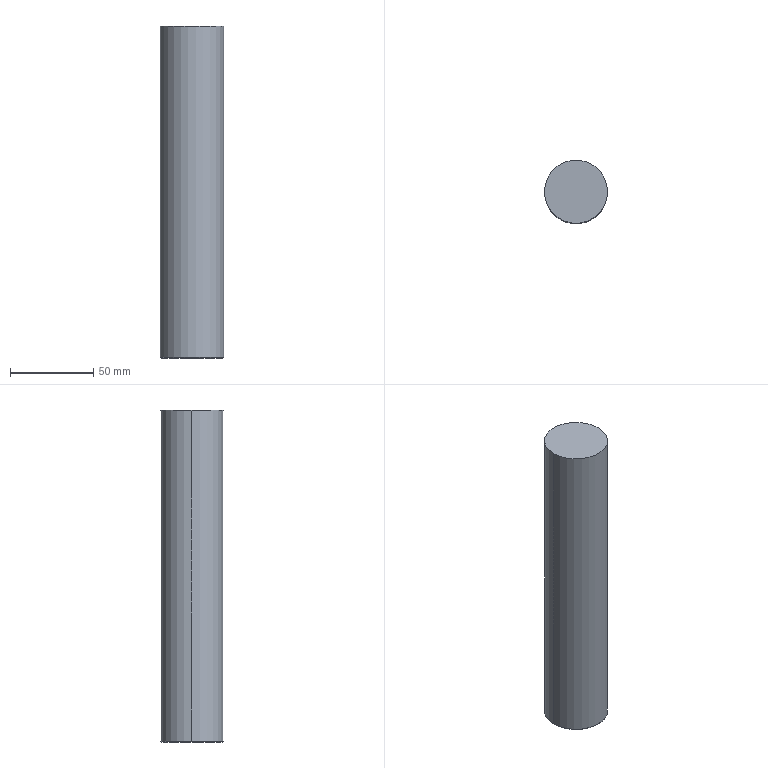Part | NX | features MYKP38-200_3 2 | 1 solid | 6 faces | box 38 x 38 x 200 mm | volume 226808 mm3 | cone 2 | plane 2 | cylinder 2 | commonest cylinder face diameters 38 x2
STEP:
#1=CARTESIAN_POINT('',(1741.477,-312.405,-150.001));
#2=VERTEX_POINT('',#1);
#3=CARTESIAN_POINT('',(1740.977,-312.405,-149.501));
#4=VERTEX_POINT('',#3);
#5=CARTESIAN_POINT('',(1741.477,-312.405,-150.001));
#6=DIRECTION('',(-0.7071,-0.000000003,0.7071));
#7=VECTOR('',#6,1000.);
#8=LINE('',#5,#7);
#9=EDGE_CURVE('',#2,#4,#8,.T.);
#10=ORIENTED_EDGE('',*,*,#9,.F.);
#11=CARTESIAN_POINT('',(1778.477,-312.405,-150.001));
#12=VERTEX_POINT('',#11);
#13=CARTESIAN_POINT('',(1759.977,-312.405,-150.001));
#14=DIRECTION('',(0.,0.,1.));
#15=DIRECTION('',(-1.,0.,0.));
#16=AXIS2_PLACEMENT_3D('',#13,#14,#15);
#17=CIRCLE('',#16,18.5);
#18=EDGE_CURVE('',#2,#12,#17,.T.);
#19=ORIENTED_EDGE('',*,*,#18,.T.);
#20=CARTESIAN_POINT('',(1778.977,-312.405,-149.501));
#21=VERTEX_POINT('',#20);
#22=CARTESIAN_POINT('',(1778.477,-312.405,-150.001));
#23=DIRECTION('',(0.7071,0.000000003,0.7071));
#24=VECTOR('',#23,1000.);
#25=LINE('',#22,#24);
#26=EDGE_CURVE('',#21,#12,#25,.F.);
#27=ORIENTED_EDGE('',*,*,#26,.F.);
#28=CARTESIAN_POINT('',(1759.977,-312.405,-149.501));
#29=DIRECTION('',(0.,0.,1.));
#30=DIRECTION('',(-1.,0.,0.));
#31=AXIS2_PLACEMENT_3D('',#28,#29,#30);
#32=CIRCLE('',#31,19.);
#33=EDGE_CURVE('',#4,#21,#32,.T.);
#34=ORIENTED_EDGE('',*,*,#33,.F.);
#35=EDGE_LOOP('',(#10,#19,#27,#34));
#36=FACE_BOUND('',#35,.T.);
#37=CARTESIAN_POINT('',(1759.977,-312.405,-149.751));
#38=DIRECTION('',(0.,0.,1.));
#39=DIRECTION('',(0.,-1.,0.));
#40=AXIS2_PLACEMENT_3D('',#37,#38,#39);
#41=CONICAL_SURFACE('',#40,18.75,0.7854);
#42=ADVANCED_FACE('',(#36),#41,.T.);
#43=ORIENTED_EDGE('',*,*,#26,.T.);
#44=CARTESIAN_POINT('',(1759.977,-312.405,-150.001));
#45=DIRECTION('',(0.,0.,1.));
#46=DIRECTION('',(1.,0.,0.));
#47=AXIS2_PLACEMENT_3D('',#44,#45,#46);
#48=CIRCLE('',#47,18.5);
#49=EDGE_CURVE('',#12,#2,#48,.T.);
#50=ORIENTED_EDGE('',*,*,#49,.T.);
#51=ORIENTED_EDGE('',*,*,#9,.T.);
#52=CARTESIAN_POINT('',(1759.977,-312.405,-149.501));
#53=DIRECTION('',(0.,0.,1.));
#54=DIRECTION('',(1.,0.,0.));
#55=AXIS2_PLACEMENT_3D('',#52,#53,#54);
#56=CIRCLE('',#55,19.);
#57=EDGE_CURVE('',#21,#4,#56,.T.);
#58=ORIENTED_EDGE('',*,*,#57,.F.);
#59=EDGE_LOOP('',(#43,#50,#51,#58));
#60=FACE_BOUND('',#59,.T.);
#61=CARTESIAN_POINT('',(1759.977,-312.405,-149.751));
#62=DIRECTION('',(0.,0.,1.));
#63=DIRECTION('',(0.,-1.,0.));
#64=AXIS2_PLACEMENT_3D('',#61,#62,#63);
#65=CONICAL_SURFACE('',#64,18.75,0.7854);
#66=ADVANCED_FACE('',(#60),#65,.T.);
#67=ORIENTED_EDGE('',*,*,#18,.F.);
#68=ORIENTED_EDGE('',*,*,#49,.F.);
#69=EDGE_LOOP('',(#67,#68));
#70=FACE_BOUND('',#69,.T.);
#71=CARTESIAN_POINT('',(1759.977,-312.405,-150.001));
#72=DIRECTION('',(0.,0.,-1.));
#73=DIRECTION('',(1.,0.,0.));
#74=AXIS2_PLACEMENT_3D('',#71,#72,#73);
#75=PLANE('',#74);
#76=ADVANCED_FACE('',(#70),#75,.T.);
#77=CARTESIAN_POINT('',(1740.977,-312.405,-3.001));
#78=VERTEX_POINT('',#77);
#79=CARTESIAN_POINT('',(1740.977,-312.405,49.999));
#80=VERTEX_POINT('',#79);
#81=CARTESIAN_POINT('',(1740.977,-312.405,-79.501));
#82=DIRECTION('',(-0.000000019,0.,1.));
#83=VECTOR('',#82,1000.);
#84=LINE('',#81,#83);
#85=EDGE_CURVE('',#78,#80,#84,.T.);
#86=ORIENTED_EDGE('',*,*,#85,.T.);
#87=CARTESIAN_POINT('',(1778.977,-312.405,49.999));
#88=VERTEX_POINT('',#87);
#89=CARTESIAN_POINT('',(1759.977,-312.405,49.999));
#90=DIRECTION('',(0.,0.,-1.));
#91=DIRECTION('',(-1.,0.,0.));
#92=AXIS2_PLACEMENT_3D('',#89,#90,#91);
#93=CIRCLE('',#92,19.);
#94=EDGE_CURVE('',#80,#88,#93,.T.);
#95=ORIENTED_EDGE('',*,*,#94,.T.);
#96=CARTESIAN_POINT('',(1778.977,-312.405,-3.001));
#97=VERTEX_POINT('',#96);
#98=CARTESIAN_POINT('',(1778.977,-312.405,-79.501));
#99=DIRECTION('',(0.000000019,0.,1.));
#100=VECTOR('',#99,1000.);
#101=LINE('',#98,#100);
#102=EDGE_CURVE('',#88,#97,#101,.F.);
#103=ORIENTED_EDGE('',*,*,#102,.T.);
#104=CARTESIAN_POINT('',(1778.977,-312.405,-5.001));
#105=VERTEX_POINT('',#104);
#106=CARTESIAN_POINT('',(1778.977,-312.405,-79.501));
#107=DIRECTION('',(0.000000019,0.,1.));
#108=VECTOR('',#107,1000.);
#109=LINE('',#106,#108);
#110=EDGE_CURVE('',#97,#105,#109,.F.);
#111=ORIENTED_EDGE('',*,*,#110,.T.);
#112=CARTESIAN_POINT('',(1778.977,-312.405,-7.001));
#113=VERTEX_POINT('',#112);
#114=CARTESIAN_POINT('',(1778.977,-312.405,-81.501));
#115=DIRECTION('',(0.000000019,0.,1.));
#116=VECTOR('',#115,1000.);
#117=LINE('',#114,#116);
#118=EDGE_CURVE('',#105,#113,#117,.F.);
#119=ORIENTED_EDGE('',*,*,#118,.T.);
#120=CARTESIAN_POINT('',(1778.977,-312.405,-9.001));
#121=VERTEX_POINT('',#120);
#122=CARTESIAN_POINT('',(1778.977,-312.405,-83.501));
#123=DIRECTION('',(0.000000019,0.,1.));
#124=VECTOR('',#123,1000.);
#125=LINE('',#122,#124);
#126=EDGE_CURVE('',#113,#121,#125,.F.);
#127=ORIENTED_EDGE('',*,*,#126,.T.);
#128=CARTESIAN_POINT('',(1778.977,-312.405,-11.001));
#129=VERTEX_POINT('',#128);
#130=CARTESIAN_POINT('',(1778.977,-312.405,-85.501));
#131=DIRECTION('',(0.000000019,0.,1.));
#132=VECTOR('',#131,1000.);
#133=LINE('',#130,#132);
#134=EDGE_CURVE('',#121,#129,#133,.F.);
#135=ORIENTED_EDGE('',*,*,#134,.T.);
#136=CARTESIAN_POINT('',(1778.977,-312.405,-13.001));
#137=VERTEX_POINT('',#136);
#138=CARTESIAN_POINT('',(1778.977,-312.405,-87.501));
#139=DIRECTION('',(0.000000019,0.,1.));
#140=VECTOR('',#139,1000.);
#141=LINE('',#138,#140);
#142=EDGE_CURVE('',#129,#137,#141,.F.);
#143=ORIENTED_EDGE('',*,*,#142,.T.);
#144=CARTESIAN_POINT('',(1778.977,-312.405,-15.001));
#145=VERTEX_POINT('',#144);
#146=CARTESIAN_POINT('',(1778.977,-312.405,-89.501));
#147=DIRECTION('',(0.000000019,0.,1.));
#148=VECTOR('',#147,1000.);
#149=LINE('',#146,#148);
#150=EDGE_CURVE('',#137,#145,#149,.F.);
#151=ORIENTED_EDGE('',*,*,#150,.T.);
#152=CARTESIAN_POINT('',(1778.977,-312.405,-17.001));
#153=VERTEX_POINT('',#152);
#154=CARTESIAN_POINT('',(1778.977,-312.405,-91.501));
#155=DIRECTION('',(0.000000019,0.,1.));
#156=VECTOR('',#155,1000.);
#157=LINE('',#154,#156);
#158=EDGE_CURVE('',#145,#153,#157,.F.);
#159=ORIENTED_EDGE('',*,*,#158,.T.);
#160=CARTESIAN_POINT('',(1778.977,-312.405,-19.001));
#161=VERTEX_POINT('',#160);
#162=CARTESIAN_POINT('',(1778.977,-312.405,-93.501));
#163=DIRECTION('',(0.000000019,0.,1.));
#164=VECTOR('',#163,1000.);
#165=LINE('',#162,#164);
#166=EDGE_CURVE('',#153,#161,#165,.F.);
#167=ORIENTED_EDGE('',*,*,#166,.T.);
#168=CARTESIAN_POINT('',(1778.977,-312.405,-21.001));
#169=VERTEX_POINT('',#168);
#170=CARTESIAN_POINT('',(1778.977,-312.405,-95.501));
#171=DIRECTION('',(0.000000019,0.,1.));
#172=VECTOR('',#171,1000.);
#173=LINE('',#170,#172);
#174=EDGE_CURVE('',#161,#169,#173,.F.);
#175=ORIENTED_EDGE('',*,*,#174,.T.);
#176=CARTESIAN_POINT('',(1778.977,-312.405,-23.001));
#177=VERTEX_POINT('',#176);
#178=CARTESIAN_POINT('',(1778.977,-312.405,-97.501));
#179=DIRECTION('',(0.000000019,0.,1.));
#180=VECTOR('',#179,1000.);
#181=LINE('',#178,#180);
#182=EDGE_CURVE('',#169,#177,#181,.F.);
#183=ORIENTED_EDGE('',*,*,#182,.T.);
#184=CARTESIAN_POINT('',(1778.977,-312.405,-25.001));
#185=VERTEX_POINT('',#184);
#186=CARTESIAN_POINT('',(1778.977,-312.405,-99.501));
#187=DIRECTION('',(0.000000019,0.,1.));
#188=VECTOR('',#187,1000.);
#189=LINE('',#186,#188);
#190=EDGE_CURVE('',#177,#185,#189,.F.);
#191=ORIENTED_EDGE('',*,*,#190,.T.);
#192=CARTESIAN_POINT('',(1778.977,-312.405,-27.001));
#193=VERTEX_POINT('',#192);
#194=CARTESIAN_POINT('',(1778.977,-312.405,-101.501));
#195=DIRECTION('',(0.000000019,0.,1.));
#196=VECTOR('',#195,1000.);
#197=LINE('',#194,#196);
#198=EDGE_CURVE('',#185,#193,#197,.F.);
#199=ORIENTED_EDGE('',*,*,#198,.T.);
#200=CARTESIAN_POINT('',(1778.977,-312.405,-29.001));
#201=VERTEX_POINT('',#200);
#202=CARTESIAN_POINT('',(1778.977,-312.405,-103.501));
#203=DIRECTION('',(0.000000019,0.,1.));
#204=VECTOR('',#203,1000.);
#205=LINE('',#202,#204);
#206=EDGE_CURVE('',#193,#201,#205,.F.);
#207=ORIENTED_EDGE('',*,*,#206,.T.);
#208=CARTESIAN_POINT('',(1778.977,-312.405,-31.001));
#209=VERTEX_POINT('',#208);
#210=CARTESIAN_POINT('',(1778.977,-312.405,-105.501));
#211=DIRECTION('',(0.000000019,0.,1.));
#212=VECTOR('',#211,1000.);
#213=LINE('',#210,#212);
#214=EDGE_CURVE('',#201,#209,#213,.F.);
#215=ORIENTED_EDGE('',*,*,#214,.T.);
#216=CARTESIAN_POINT('',(1778.977,-312.405,-33.001));
#217=VERTEX_POINT('',#216);
#218=CARTESIAN_POINT('',(1778.977,-312.405,-107.501));
#219=DIRECTION('',(0.000000019,0.,1.));
#220=VECTOR('',#219,1000.);
#221=LINE('',#218,#220);
#222=EDGE_CURVE('',#209,#217,#221,.F.);
#223=ORIENTED_EDGE('',*,*,#222,.T.);
#224=CARTESIAN_POINT('',(1778.977,-312.405,-35.001));
#225=VERTEX_POINT('',#224);
#226=CARTESIAN_POINT('',(1778.977,-312.405,-109.501));
#227=DIRECTION('',(0.000000019,0.,1.));
#228=VECTOR('',#227,1000.);
#229=LINE('',#226,#228);
#230=EDGE_CURVE('',#217,#225,#229,.F.);
#231=ORIENTED_EDGE('',*,*,#230,.T.);
#232=CARTESIAN_POINT('',(1778.977,-312.405,-37.001));
#233=VERTEX_POINT('',#232);
#234=CARTESIAN_POINT('',(1778.977,-312.405,-111.501));
#235=DIRECTION('',(0.000000019,0.,1.));
#236=VECTOR('',#235,1000.);
#237=LINE('',#234,#236);
#238=EDGE_CURVE('',#225,#233,#237,.F.);
#239=ORIENTED_EDGE('',*,*,#238,.T.);
#240=CARTESIAN_POINT('',(1778.977,-312.405,-39.001));
#241=VERTEX_POINT('',#240);
#242=CARTESIAN_POINT('',(1778.977,-312.405,-113.501));
#243=DIRECTION('',(0.000000019,0.,1.));
#244=VECTOR('',#243,1000.);
#245=LINE('',#242,#244);
#246=EDGE_CURVE('',#233,#241,#245,.F.);
#247=ORIENTED_EDGE('',*,*,#246,.T.);
#248=CARTESIAN_POINT('',(1778.977,-312.405,-41.001));
#249=VERTEX_POINT('',#248);
#250=CARTESIAN_POINT('',(1778.977,-312.405,-115.501));
#251=DIRECTION('',(0.000000019,0.,1.));
#252=VECTOR('',#251,1000.);
#253=LINE('',#250,#252);
#254=EDGE_CURVE('',#241,#249,#253,.F.);
#255=ORIENTED_EDGE('',*,*,#254,.T.);
#256=CARTESIAN_POINT('',(1778.977,-312.405,-43.001));
#257=VERTEX_POINT('',#256);
#258=CARTESIAN_POINT('',(1778.977,-312.405,-117.501));
#259=DIRECTION('',(0.000000019,0.,1.));
#260=VECTOR('',#259,1000.);
#261=LINE('',#258,#260);
#262=EDGE_CURVE('',#249,#257,#261,.F.);
#263=ORIENTED_EDGE('',*,*,#262,.T.);
#264=CARTESIAN_POINT('',(1778.977,-312.405,-45.001));
#265=VERTEX_POINT('',#264);
#266=CARTESIAN_POINT('',(1778.977,-312.405,-119.501));
#267=DIRECTION('',(0.000000019,0.,1.));
#268=VECTOR('',#267,1000.);
#269=LINE('',#266,#268);
#270=EDGE_CURVE('',#257,#265,#269,.F.);
#271=ORIENTED_EDGE('',*,*,#270,.T.);
#272=CARTESIAN_POINT('',(1778.977,-312.405,-47.001));
#273=VERTEX_POINT('',#272);
#274=CARTESIAN_POINT('',(1778.977,-312.405,-121.501));
#275=DIRECTION('',(0.000000019,0.,1.));
#276=VECTOR('',#275,1000.);
#277=LINE('',#274,#276);
#278=EDGE_CURVE('',#265,#273,#277,.F.);
#279=ORIENTED_EDGE('',*,*,#278,.T.);
#280=CARTESIAN_POINT('',(1778.977,-312.405,-49.001));
#281=VERTEX_POINT('',#280);
#282=CARTESIAN_POINT('',(1778.977,-312.405,-123.501));
#283=DIRECTION('',(0.000000019,0.,1.));
#284=VECTOR('',#283,1000.);
#285=LINE('',#282,#284);
#286=EDGE_CURVE('',#273,#281,#285,.F.);
#287=ORIENTED_EDGE('',*,*,#286,.T.);
#288=CARTESIAN_POINT('',(1778.977,-312.405,-51.001));
#289=VERTEX_POINT('',#288);
#290=CARTESIAN_POINT('',(1778.977,-312.405,-125.501));
#291=DIRECTION('',(0.000000019,0.,1.));
#292=VECTOR('',#291,1000.);
#293=LINE('',#290,#292);
#294=EDGE_CURVE('',#281,#289,#293,.F.);
#295=ORIENTED_EDGE('',*,*,#294,.T.);
#296=CARTESIAN_POINT('',(1778.977,-312.405,-53.001));
#297=VERTEX_POINT('',#296);
#298=CARTESIAN_POINT('',(1778.977,-312.405,-127.501));
#299=DIRECTION('',(0.000000019,0.,1.));
#300=VECTOR('',#299,1000.);
#301=LINE('',#298,#300);
#302=EDGE_CURVE('',#289,#297,#301,.F.);
#303=ORIENTED_EDGE('',*,*,#302,.T.);
#304=CARTESIAN_POINT('',(1778.977,-312.405,-55.001));
#305=VERTEX_POINT('',#304);
#306=CARTESIAN_POINT('',(1778.977,-312.405,-129.501));
#307=DIRECTION('',(0.000000019,0.,1.));
#308=VECTOR('',#307,1000.);
#309=LINE('',#306,#308);
#310=EDGE_CURVE('',#297,#305,#309,.F.);
#311=ORIENTED_EDGE('',*,*,#310,.T.);
#312=CARTESIAN_POINT('',(1778.977,-312.405,-57.001));
#313=VERTEX_POINT('',#312);
#314=CARTESIAN_POINT('',(1778.977,-312.405,-131.501));
#315=DIRECTION('',(0.000000019,0.,1.));
#316=VECTOR('',#315,1000.);
#317=LINE('',#314,#316);
#318=EDGE_CURVE('',#305,#313,#317,.F.);
#319=ORIENTED_EDGE('',*,*,#318,.T.);
#320=CARTESIAN_POINT('',(1778.977,-312.405,-59.001));
#321=VERTEX_POINT('',#320);
#322=CARTESIAN_POINT('',(1778.977,-312.405,-133.501));
#323=DIRECTION('',(0.000000019,0.,1.));
#324=VECTOR('',#323,1000.);
#325=LINE('',#322,#324);
#326=EDGE_CURVE('',#313,#321,#325,.F.);
#327=ORIENTED_EDGE('',*,*,#326,.T.);
#328=CARTESIAN_POINT('',(1778.977,-312.405,-61.001));
#329=VERTEX_POINT('',#328);
#330=CARTESIAN_POINT('',(1778.977,-312.405,-135.501));
#331=DIRECTION('',(0.000000019,0.,1.));
#332=VECTOR('',#331,1000.);
#333=LINE('',#330,#332);
#334=EDGE_CURVE('',#321,#329,#333,.F.);
#335=ORIENTED_EDGE('',*,*,#334,.T.);
#336=CARTESIAN_POINT('',(1778.977,-312.405,-63.001));
#337=VERTEX_POINT('',#336);
#338=CARTESIAN_POINT('',(1778.977,-312.405,-137.501));
#339=DIRECTION('',(0.000000019,0.,1.));
#340=VECTOR('',#339,1000.);
#341=LINE('',#338,#340);
#342=EDGE_CURVE('',#329,#337,#341,.F.);
#343=ORIENTED_EDGE('',*,*,#342,.T.);
#344=CARTESIAN_POINT('',(1778.977,-312.405,-65.001));
#345=VERTEX_POINT('',#344);
#346=CARTESIAN_POINT('',(1778.977,-312.405,-139.501));
#347=DIRECTION('',(0.000000019,0.,1.));
#348=VECTOR('',#347,1000.);
#349=LINE('',#346,#348);
#350=EDGE_CURVE('',#337,#345,#349,.F.);
#351=ORIENTED_EDGE('',*,*,#350,.T.);
#352=CARTESIAN_POINT('',(1778.977,-312.405,-67.001));
#353=VERTEX_POINT('',#352);
#354=CARTESIAN_POINT('',(1778.977,-312.405,-141.501));
#355=DIRECTION('',(0.000000019,0.,1.));
#356=VECTOR('',#355,1000.);
#357=LINE('',#354,#356);
#358=EDGE_CURVE('',#345,#353,#357,.F.);
#359=ORIENTED_EDGE('',*,*,#358,.T.);
#360=CARTESIAN_POINT('',(1778.977,-312.405,-69.001));
#361=VERTEX_POINT('',#360);
#362=CARTESIAN_POINT('',(1778.977,-312.405,-143.501));
#363=DIRECTION('',(0.000000019,0.,1.));
#364=VECTOR('',#363,1000.);
#365=LINE('',#362,#364);
#366=EDGE_CURVE('',#353,#361,#365,.F.);
#367=ORIENTED_EDGE('',*,*,#366,.T.);
#368=CARTESIAN_POINT('',(1778.977,-312.405,-71.001));
#369=VERTEX_POINT('',#368);
#370=CARTESIAN_POINT('',(1778.977,-312.405,-145.501));
#371=DIRECTION('',(0.000000019,0.,1.));
#372=VECTOR('',#371,1000.);
#373=LINE('',#370,#372);
#374=EDGE_CURVE('',#361,#369,#373,.F.);
#375=ORIENTED_EDGE('',*,*,#374,.T.);
#376=CARTESIAN_POINT('',(1778.977,-312.405,-73.001));
#377=VERTEX_POINT('',#376);
#378=CARTESIAN_POINT('',(1778.977,-312.405,-147.501));
#379=DIRECTION('',(0.000000019,0.,1.));
#380=VECTOR('',#379,1000.);
#381=LINE('',#378,#380);
#382=EDGE_CURVE('',#369,#377,#381,.F.);
#383=ORIENTED_EDGE('',*,*,#382,.T.);
#384=CARTESIAN_POINT('',(1778.977,-312.405,-75.001));
#385=VERTEX_POINT('',#384);
#386=CARTESIAN_POINT('',(1778.977,-312.405,-149.501));
#387=DIRECTION('',(0.000000019,0.,1.));
#388=VECTOR('',#387,1000.);
#389=LINE('',#386,#388);
#390=EDGE_CURVE('',#377,#385,#389,.F.);
#391=ORIENTED_EDGE('',*,*,#390,.T.);
#392=CARTESIAN_POINT('',(1778.977,-312.405,-149.501));
#393=DIRECTION('',(0.000000019,0.,1.));
#394=VECTOR('',#393,1000.);
#395=LINE('',#392,#394);
#396=EDGE_CURVE('',#385,#21,#395,.F.);
#397=ORIENTED_EDGE('',*,*,#396,.T.);
#398=ORIENTED_EDGE('',*,*,#57,.T.);
#399=CARTESIAN_POINT('',(1740.977,-312.405,-75.001));
#400=VERTEX_POINT('',#399);
#401=CARTESIAN_POINT('',(1740.977,-312.405,-149.501));
#402=DIRECTION('',(-0.000000019,0.,1.));
#403=VECTOR('',#402,1000.);
#404=LINE('',#401,#403);
#405=EDGE_CURVE('',#4,#400,#404,.T.);
#406=ORIENTED_EDGE('',*,*,#405,.T.);
#407=CARTESIAN_POINT('',(1740.977,-312.405,-73.001));
#408=VERTEX_POINT('',#407);
#409=CARTESIAN_POINT('',(1740.977,-312.405,-149.501));
#410=DIRECTION('',(-0.000000019,0.,1.));
#411=VECTOR('',#410,1000.);
#412=LINE('',#409,#411);
#413=EDGE_CURVE('',#400,#408,#412,.T.);
#414=ORIENTED_EDGE('',*,*,#413,.T.);
#415=CARTESIAN_POINT('',(1740.977,-312.405,-71.001));
#416=VERTEX_POINT('',#415);
#417=CARTESIAN_POINT('',(1740.977,-312.405,-147.501));
#418=DIRECTION('',(-0.000000019,0.,1.));
#419=VECTOR('',#418,1000.);
#420=LINE('',#417,#419);
#421=EDGE_CURVE('',#408,#416,#420,.T.);
#422=ORIENTED_EDGE('',*,*,#421,.T.);
#423=CARTESIAN_POINT('',(1740.977,-312.405,-69.001));
#424=VERTEX_POINT('',#423);
#425=CARTESIAN_POINT('',(1740.977,-312.405,-145.501));
#426=DIRECTION('',(-0.000000019,0.,1.));
#427=VECTOR('',#426,1000.);
#428=LINE('',#425,#427);
#429=EDGE_CURVE('',#416,#424,#428,.T.);
#430=ORIENTED_EDGE('',*,*,#429,.T.);
#431=CARTESIAN_POINT('',(1740.977,-312.405,-67.001));
#432=VERTEX_POINT('',#431);
#433=CARTESIAN_POINT('',(1740.977,-312.405,-143.501));
#434=DIRECTION('',(-0.000000019,0.,1.));
#435=VECTOR('',#434,1000.);
#436=LINE('',#433,#435);
#437=EDGE_CURVE('',#424,#432,#436,.T.);
#438=ORIENTED_EDGE('',*,*,#437,.T.);
#439=CARTESIAN_POINT('',(1740.977,-312.405,-65.001));
#440=VERTEX_POINT('',#439);
#441=CARTESIAN_POINT('',(1740.977,-312.405,-141.501));
#442=DIRECTION('',(-0.000000019,0.,1.));
#443=VECTOR('',#442,1000.);
#444=LINE('',#441,#443);
#445=EDGE_CURVE('',#432,#440,#444,.T.);
#446=ORIENTED_EDGE('',*,*,#445,.T.);
#447=CARTESIAN_POINT('',(1740.977,-312.405,-63.001));
#448=VERTEX_POINT('',#447);
#449=CARTESIAN_POINT('',(1740.977,-312.405,-139.501));
#450=DIRECTION('',(-0.000000019,0.,1.));
#451=VECTOR('',#450,1000.);
#452=LINE('',#449,#451);
#453=EDGE_CURVE('',#440,#448,#452,.T.);
#454=ORIENTED_EDGE('',*,*,#453,.T.);
#455=CARTESIAN_POINT('',(1740.977,-312.405,-61.001));
#456=VERTEX_POINT('',#455);
#457=CARTESIAN_POINT('',(1740.977,-312.405,-137.501));
#458=DIRECTION('',(-0.000000019,0.,1.));
#459=VECTOR('',#458,1000.);
#460=LINE('',#457,#459);
#461=EDGE_CURVE('',#448,#456,#460,.T.);
#462=ORIENTED_EDGE('',*,*,#461,.T.);
#463=CARTESIAN_POINT('',(1740.977,-312.405,-59.001));
#464=VERTEX_POINT('',#463);
#465=CARTESIAN_POINT('',(1740.977,-312.405,-135.501));
#466=DIRECTION('',(-0.000000019,0.,1.));
#467=VECTOR('',#466,1000.);
#468=LINE('',#465,#467);
#469=EDGE_CURVE('',#456,#464,#468,.T.);
#470=ORIENTED_EDGE('',*,*,#469,.T.);
#471=CARTESIAN_POINT('',(1740.977,-312.405,-57.001));
#472=VERTEX_POINT('',#471);
#473=CARTESIAN_POINT('',(1740.977,-312.405,-133.501));
#474=DIRECTION('',(-0.000000019,0.,1.));
#475=VECTOR('',#474,1000.);
#476=LINE('',#473,#475);
#477=EDGE_CURVE('',#464,#472,#476,.T.);
#478=ORIENTED_EDGE('',*,*,#477,.T.);
#479=CARTESIAN_POINT('',(1740.977,-312.405,-55.001));
#480=VERTEX_POINT('',#479);
#481=CARTESIAN_POINT('',(1740.977,-312.405,-131.501));
#482=DIRECTION('',(-0.000000019,0.,1.));
#483=VECTOR('',#482,1000.);
#484=LINE('',#481,#483);
#485=EDGE_CURVE('',#472,#480,#484,.T.);
#486=ORIENTED_EDGE('',*,*,#485,.T.);
#487=CARTESIAN_POINT('',(1740.977,-312.405,-53.001));
#488=VERTEX_POINT('',#487);
#489=CARTESIAN_POINT('',(1740.977,-312.405,-129.501));
#490=DIRECTION('',(-0.000000019,0.,1.));
#491=VECTOR('',#490,1000.);
#492=LINE('',#489,#491);
#493=EDGE_CURVE('',#480,#488,#492,.T.);
#494=ORIENTED_EDGE('',*,*,#493,.T.);
#495=CARTESIAN_POINT('',(1740.977,-312.405,-51.001));
#496=VERTEX_POINT('',#495);
#497=CARTESIAN_POINT('',(1740.977,-312.405,-127.501));
#498=DIRECTION('',(-0.000000019,0.,1.));
#499=VECTOR('',#498,1000.);
#500=LINE('',#497,#499);
#501=EDGE_CURVE('',#488,#496,#500,.T.);
#502=ORIENTED_EDGE('',*,*,#501,.T.);
#503=CARTESIAN_POINT('',(1740.977,-312.405,-49.001));
#504=VERTEX_POINT('',#503);
#505=CARTESIAN_POINT('',(1740.977,-312.405,-125.501));
#506=DIRECTION('',(-0.000000019,0.,1.));
#507=VECTOR('',#506,1000.);
#508=LINE('',#505,#507);
#509=EDGE_CURVE('',#496,#504,#508,.T.);
#510=ORIENTED_EDGE('',*,*,#509,.T.);
#511=CARTESIAN_POINT('',(1740.977,-312.405,-47.001));
#512=VERTEX_POINT('',#511);
#513=CARTESIAN_POINT('',(1740.977,-312.405,-123.501));
#514=DIRECTION('',(-0.000000019,0.,1.));
#515=VECTOR('',#514,1000.);
#516=LINE('',#513,#515);
#517=EDGE_CURVE('',#504,#512,#516,.T.);
#518=ORIENTED_EDGE('',*,*,#517,.T.);
#519=CARTESIAN_POINT('',(1740.977,-312.405,-45.001));
#520=VERTEX_POINT('',#519);
#521=CARTESIAN_POINT('',(1740.977,-312.405,-121.501));
#522=DIRECTION('',(-0.000000019,0.,1.));
#523=VECTOR('',#522,1000.);
#524=LINE('',#521,#523);
#525=EDGE_CURVE('',#512,#520,#524,.T.);
#526=ORIENTED_EDGE('',*,*,#525,.T.);
#527=CARTESIAN_POINT('',(1740.977,-312.405,-43.001));
#528=VERTEX_POINT('',#527);
#529=CARTESIAN_POINT('',(1740.977,-312.405,-119.501));
#530=DIRECTION('',(-0.000000019,0.,1.));
#531=VECTOR('',#530,1000.);
#532=LINE('',#529,#531);
#533=EDGE_CURVE('',#520,#528,#532,.T.);
#534=ORIENTED_EDGE('',*,*,#533,.T.);
#535=CARTESIAN_POINT('',(1740.977,-312.405,-41.001));
#536=VERTEX_POINT('',#535);
#537=CARTESIAN_POINT('',(1740.977,-312.405,-117.501));
#538=DIRECTION('',(-0.000000019,0.,1.));
#539=VECTOR('',#538,1000.);
#540=LINE('',#537,#539);
#541=EDGE_CURVE('',#528,#536,#540,.T.);
#542=ORIENTED_EDGE('',*,*,#541,.T.);
#543=CARTESIAN_POINT('',(1740.977,-312.405,-39.001));
#544=VERTEX_POINT('',#543);
#545=CARTESIAN_POINT('',(1740.977,-312.405,-115.501));
#546=DIRECTION('',(-0.000000019,0.,1.));
#547=VECTOR('',#546,1000.);
#548=LINE('',#545,#547);
#549=EDGE_CURVE('',#536,#544,#548,.T.);
#550=ORIENTED_EDGE('',*,*,#549,.T.);
#551=CARTESIAN_POINT('',(1740.977,-312.405,-37.001));
#552=VERTEX_POINT('',#551);
#553=CARTESIAN_POINT('',(1740.977,-312.405,-113.501));
#554=DIRECTION('',(-0.000000019,0.,1.));
#555=VECTOR('',#554,1000.);
#556=LINE('',#553,#555);
#557=EDGE_CURVE('',#544,#552,#556,.T.);
#558=ORIENTED_EDGE('',*,*,#557,.T.);
#559=CARTESIAN_POINT('',(1740.977,-312.405,-35.001));
#560=VERTEX_POINT('',#559);
#561=CARTESIAN_POINT('',(1740.977,-312.405,-111.501));
#562=DIRECTION('',(-0.000000019,0.,1.));
#563=VECTOR('',#562,1000.);
#564=LINE('',#561,#563);
#565=EDGE_CURVE('',#552,#560,#564,.T.);
#566=ORIENTED_EDGE('',*,*,#565,.T.);
#567=CARTESIAN_POINT('',(1740.977,-312.405,-33.001));
#568=VERTEX_POINT('',#567);
#569=CARTESIAN_POINT('',(1740.977,-312.405,-109.501));
#570=DIRECTION('',(-0.000000019,0.,1.));
#571=VECTOR('',#570,1000.);
#572=LINE('',#569,#571);
#573=EDGE_CURVE('',#560,#568,#572,.T.);
#574=ORIENTED_EDGE('',*,*,#573,.T.);
#575=CARTESIAN_POINT('',(1740.977,-312.405,-31.001));
#576=VERTEX_POINT('',#575);
#577=CARTESIAN_POINT('',(1740.977,-312.405,-107.501));
#578=DIRECTION('',(-0.000000019,0.,1.));
#579=VECTOR('',#578,1000.);
#580=LINE('',#577,#579);
#581=EDGE_CURVE('',#568,#576,#580,.T.);
#582=ORIENTED_EDGE('',*,*,#581,.T.);
#583=CARTESIAN_POINT('',(1740.977,-312.405,-29.001));
#584=VERTEX_POINT('',#583);
#585=CARTESIAN_POINT('',(1740.977,-312.405,-105.501));
#586=DIRECTION('',(-0.000000019,0.,1.));
#587=VECTOR('',#586,1000.);
#588=LINE('',#585,#587);
#589=EDGE_CURVE('',#576,#584,#588,.T.);
#590=ORIENTED_EDGE('',*,*,#589,.T.);
#591=CARTESIAN_POINT('',(1740.977,-312.405,-27.001));
#592=VERTEX_POINT('',#591);
#593=CARTESIAN_POINT('',(1740.977,-312.405,-103.501));
#594=DIRECTION('',(-0.000000019,0.,1.));
#595=VECTOR('',#594,1000.);
#596=LINE('',#593,#595);
#597=EDGE_CURVE('',#584,#592,#596,.T.);
#598=ORIENTED_EDGE('',*,*,#597,.T.);
#599=CARTESIAN_POINT('',(1740.977,-312.405,-25.001));
#600=VERTEX_POINT('',#599);
#601=CARTESIAN_POINT('',(1740.977,-312.405,-101.501));
#602=DIRECTION('',(-0.000000019,0.,1.));
#603=VECTOR('',#602,1000.);
#604=LINE('',#601,#603);
#605=EDGE_CURVE('',#592,#600,#604,.T.);
#606=ORIENTED_EDGE('',*,*,#605,.T.);
#607=CARTESIAN_POINT('',(1740.977,-312.405,-23.001));
#608=VERTEX_POINT('',#607);
#609=CARTESIAN_POINT('',(1740.977,-312.405,-99.501));
#610=DIRECTION('',(-0.000000019,0.,1.));
#611=VECTOR('',#610,1000.);
#612=LINE('',#609,#611);
#613=EDGE_CURVE('',#600,#608,#612,.T.);
#614=ORIENTED_EDGE('',*,*,#613,.T.);
#615=CARTESIAN_POINT('',(1740.977,-312.405,-21.001));
#616=VERTEX_POINT('',#615);
#617=CARTESIAN_POINT('',(1740.977,-312.405,-97.501));
#618=DIRECTION('',(-0.000000019,0.,1.));
#619=VECTOR('',#618,1000.);
#620=LINE('',#617,#619);
#621=EDGE_CURVE('',#608,#616,#620,.T.);
#622=ORIENTED_EDGE('',*,*,#621,.T.);
#623=CARTESIAN_POINT('',(1740.977,-312.405,-19.001));
#624=VERTEX_POINT('',#623);
#625=CARTESIAN_POINT('',(1740.977,-312.405,-95.501));
#626=DIRECTION('',(-0.000000019,0.,1.));
#627=VECTOR('',#626,1000.);
#628=LINE('',#625,#627);
#629=EDGE_CURVE('',#616,#624,#628,.T.);
#630=ORIENTED_EDGE('',*,*,#629,.T.);
#631=CARTESIAN_POINT('',(1740.977,-312.405,-17.001));
#632=VERTEX_POINT('',#631);
#633=CARTESIAN_POINT('',(1740.977,-312.405,-93.501));
#634=DIRECTION('',(-0.000000019,0.,1.));
#635=VECTOR('',#634,1000.);
#636=LINE('',#633,#635);
#637=EDGE_CURVE('',#624,#632,#636,.T.);
#638=ORIENTED_EDGE('',*,*,#637,.T.);
#639=CARTESIAN_POINT('',(1740.977,-312.405,-15.001));
#640=VERTEX_POINT('',#639);
#641=CARTESIAN_POINT('',(1740.977,-312.405,-91.501));
#642=DIRECTION('',(-0.000000019,0.,1.));
#643=VECTOR('',#642,1000.);
#644=LINE('',#641,#643);
#645=EDGE_CURVE('',#632,#640,#644,.T.);
#646=ORIENTED_EDGE('',*,*,#645,.T.);
#647=CARTESIAN_POINT('',(1740.977,-312.405,-13.001));
#648=VERTEX_POINT('',#647);
#649=CARTESIAN_POINT('',(1740.977,-312.405,-89.501));
#650=DIRECTION('',(-0.000000019,0.,1.));
#651=VECTOR('',#650,1000.);
#652=LINE('',#649,#651);
#653=EDGE_CURVE('',#640,#648,#652,.T.);
#654=ORIENTED_EDGE('',*,*,#653,.T.);
#655=CARTESIAN_POINT('',(1740.977,-312.405,-11.001));
#656=VERTEX_POINT('',#655);
#657=CARTESIAN_POINT('',(1740.977,-312.405,-87.501));
#658=DIRECTION('',(-0.000000019,0.,1.));
#659=VECTOR('',#658,1000.);
#660=LINE('',#657,#659);
#661=EDGE_CURVE('',#648,#656,#660,.T.);
#662=ORIENTED_EDGE('',*,*,#661,.T.);
#663=CARTESIAN_POINT('',(1740.977,-312.405,-9.001));
#664=VERTEX_POINT('',#663);
#665=CARTESIAN_POINT('',(1740.977,-312.405,-85.501));
#666=DIRECTION('',(-0.000000019,0.,1.));
#667=VECTOR('',#666,1000.);
#668=LINE('',#665,#667);
#669=EDGE_CURVE('',#656,#664,#668,.T.);
#670=ORIENTED_EDGE('',*,*,#669,.T.);
#671=CARTESIAN_POINT('',(1740.977,-312.405,-7.001));
#672=VERTEX_POINT('',#671);
#673=CARTESIAN_POINT('',(1740.977,-312.405,-83.501));
#674=DIRECTION('',(-0.000000019,0.,1.));
#675=VECTOR('',#674,1000.);
#676=LINE('',#673,#675);
#677=EDGE_CURVE('',#664,#672,#676,.T.);
#678=ORIENTED_EDGE('',*,*,#677,.T.);
#679=CARTESIAN_POINT('',(1740.977,-312.405,-5.001));
#680=VERTEX_POINT('',#679);
#681=CARTESIAN_POINT('',(1740.977,-312.405,-81.501));
#682=DIRECTION('',(-0.000000019,0.,1.));
#683=VECTOR('',#682,1000.);
#684=LINE('',#681,#683);
#685=EDGE_CURVE('',#672,#680,#684,.T.);
#686=ORIENTED_EDGE('',*,*,#685,.T.);
#687=CARTESIAN_POINT('',(1740.977,-312.405,-79.501));
#688=DIRECTION('',(-0.000000019,0.,1.));
#689=VECTOR('',#688,1000.);
#690=LINE('',#687,#689);
#691=EDGE_CURVE('',#680,#78,#690,.T.);
#692=ORIENTED_EDGE('',*,*,#691,.T.);
#693=EDGE_LOOP('',(#86,#95,#103,#111,#119,#127,#135,#143,#151,#159,#167,#175,#183,#191,#199,#207,#215,#223,#231,#239,#247,#255,#263,#271,#279,#287,#295,#303,#311,#319,#327,#335,#343,#351,#359,#367,#375,#383,#391,#397,#398,#406,#414,#422,#430,#438,#446,#454,#462,#470,#478,#486,#494,#502,#510,#518,#526,#534,#542,#550,#558,#566,#574,#582,#590,#598,#606,#614,#622,#630,#638,#646,#654,#662,#670,#678,#686,#692));
#694=FACE_BOUND('',#693,.T.);
#695=CARTESIAN_POINT('',(1759.977,-312.405,-80.001));
#696=DIRECTION('',(0.,0.,-1.));
#697=DIRECTION('',(-1.,0.,0.));
#698=AXIS2_PLACEMENT_3D('',#695,#696,#697);
#699=CYLINDRICAL_SURFACE('',#698,19.);
#700=ADVANCED_FACE('',(#694),#699,.T.);
#701=ORIENTED_EDGE('',*,*,#94,.F.);
#702=CARTESIAN_POINT('',(1759.977,-312.405,49.999));
#703=DIRECTION('',(0.,0.,-1.));
#704=DIRECTION('',(1.,0.,0.));
#705=AXIS2_PLACEMENT_3D('',#702,#703,#704);
#706=CIRCLE('',#705,19.);
#707=EDGE_CURVE('',#88,#80,#706,.T.);
#708=ORIENTED_EDGE('',*,*,#707,.F.);
#709=EDGE_LOOP('',(#701,#708));
#710=FACE_BOUND('',#709,.T.);
#711=CARTESIAN_POINT('',(1821.977,-349.905,49.999));
#712=DIRECTION('',(0.,0.,1.));
#713=DIRECTION('',(0.,-1.,0.));
#714=AXIS2_PLACEMENT_3D('',#711,#712,#713);
#715=PLANE('',#714);
#716=ADVANCED_FACE('',(#710),#715,.T.);
#717=ORIENTED_EDGE('',*,*,#102,.F.);
#718=ORIENTED_EDGE('',*,*,#707,.T.);
#719=ORIENTED_EDGE('',*,*,#85,.F.);
#720=ORIENTED_EDGE('',*,*,#691,.F.);
#721=ORIENTED_EDGE('',*,*,#685,.F.);
#722=ORIENTED_EDGE('',*,*,#677,.F.);
#723=ORIENTED_EDGE('',*,*,#669,.F.);
#724=ORIENTED_EDGE('',*,*,#661,.F.);
#725=ORIENTED_EDGE('',*,*,#653,.F.);
#726=ORIENTED_EDGE('',*,*,#645,.F.);
#727=ORIENTED_EDGE('',*,*,#637,.F.);
#728=ORIENTED_EDGE('',*,*,#629,.F.);
#729=ORIENTED_EDGE('',*,*,#621,.F.);
#730=ORIENTED_EDGE('',*,*,#613,.F.);
#731=ORIENTED_EDGE('',*,*,#605,.F.);
#732=ORIENTED_EDGE('',*,*,#597,.F.);
#733=ORIENTED_EDGE('',*,*,#589,.F.);
#734=ORIENTED_EDGE('',*,*,#581,.F.);
#735=ORIENTED_EDGE('',*,*,#573,.F.);
#736=ORIENTED_EDGE('',*,*,#565,.F.);
#737=ORIENTED_EDGE('',*,*,#557,.F.);
#738=ORIENTED_EDGE('',*,*,#549,.F.);
#739=ORIENTED_EDGE('',*,*,#541,.F.);
#740=ORIENTED_EDGE('',*,*,#533,.F.);
#741=ORIENTED_EDGE('',*,*,#525,.F.);
#742=ORIENTED_EDGE('',*,*,#517,.F.);
#743=ORIENTED_EDGE('',*,*,#509,.F.);
#744=ORIENTED_EDGE('',*,*,#501,.F.);
#745=ORIENTED_EDGE('',*,*,#493,.F.);
#746=ORIENTED_EDGE('',*,*,#485,.F.);
#747=ORIENTED_EDGE('',*,*,#477,.F.);
#748=ORIENTED_EDGE('',*,*,#469,.F.);
#749=ORIENTED_EDGE('',*,*,#461,.F.);
#750=ORIENTED_EDGE('',*,*,#453,.F.);
#751=ORIENTED_EDGE('',*,*,#445,.F.);
#752=ORIENTED_EDGE('',*,*,#437,.F.);
#753=ORIENTED_EDGE('',*,*,#429,.F.);
#754=ORIENTED_EDGE('',*,*,#421,.F.);
#755=ORIENTED_EDGE('',*,*,#413,.F.);
#756=ORIENTED_EDGE('',*,*,#405,.F.);
#757=ORIENTED_EDGE('',*,*,#33,.T.);
#758=ORIENTED_EDGE('',*,*,#396,.F.);
#759=ORIENTED_EDGE('',*,*,#390,.F.);
#760=ORIENTED_EDGE('',*,*,#382,.F.);
#761=ORIENTED_EDGE('',*,*,#374,.F.);
#762=ORIENTED_EDGE('',*,*,#366,.F.);
#763=ORIENTED_EDGE('',*,*,#358,.F.);
#764=ORIENTED_EDGE('',*,*,#350,.F.);
#765=ORIENTED_EDGE('',*,*,#342,.F.);
#766=ORIENTED_EDGE('',*,*,#334,.F.);
#767=ORIENTED_EDGE('',*,*,#326,.F.);
#768=ORIENTED_EDGE('',*,*,#318,.F.);
#769=ORIENTED_EDGE('',*,*,#310,.F.);
#770=ORIENTED_EDGE('',*,*,#302,.F.);
#771=ORIENTED_EDGE('',*,*,#294,.F.);
#772=ORIENTED_EDGE('',*,*,#286,.F.);
#773=ORIENTED_EDGE('',*,*,#278,.F.);
#774=ORIENTED_EDGE('',*,*,#270,.F.);
#775=ORIENTED_EDGE('',*,*,#262,.F.);
#776=ORIENTED_EDGE('',*,*,#254,.F.);
#777=ORIENTED_EDGE('',*,*,#246,.F.);
#778=ORIENTED_EDGE('',*,*,#238,.F.);
#779=ORIENTED_EDGE('',*,*,#230,.F.);
#780=ORIENTED_EDGE('',*,*,#222,.F.);
#781=ORIENTED_EDGE('',*,*,#214,.F.);
#782=ORIENTED_EDGE('',*,*,#206,.F.);
#783=ORIENTED_EDGE('',*,*,#198,.F.);
#784=ORIENTED_EDGE('',*,*,#190,.F.);
#785=ORIENTED_EDGE('',*,*,#182,.F.);
#786=ORIENTED_EDGE('',*,*,#174,.F.);
#787=ORIENTED_EDGE('',*,*,#166,.F.);
#788=ORIENTED_EDGE('',*,*,#158,.F.);
#789=ORIENTED_EDGE('',*,*,#150,.F.);
#790=ORIENTED_EDGE('',*,*,#142,.F.);
#791=ORIENTED_EDGE('',*,*,#134,.F.);
#792=ORIENTED_EDGE('',*,*,#126,.F.);
#793=ORIENTED_EDGE('',*,*,#118,.F.);
#794=ORIENTED_EDGE('',*,*,#110,.F.);
#795=EDGE_LOOP('',(#717,#718,#719,#720,#721,#722,#723,#724,#725,#726,#727,#728,#729,#730,#731,#732,#733,#734,#735,#736,#737,#738,#739,#740,#741,#742,#743,#744,#745,#746,#747,#748,#749,#750,#751,#752,#753,#754,#755,#756,#757,#758,#759,#760,#761,#762,#763,#764,#765,#766,#767,#768,#769,#770,#771,#772,#773,#774,#775,#776,#777,#778,#779,#780,#781,#782,#783,#784,#785,#786,#787,#788,#789,#790,#791,#792,#793,#794));
#796=FACE_BOUND('',#795,.T.);
#797=CARTESIAN_POINT('',(1759.977,-312.405,-80.001));
#798=DIRECTION('',(0.,0.,-1.));
#799=DIRECTION('',(-1.,0.,0.));
#800=AXIS2_PLACEMENT_3D('',#797,#798,#799);
#801=CYLINDRICAL_SURFACE('',#800,19.);
#802=ADVANCED_FACE('',(#796),#801,.T.);
#803=CLOSED_SHELL('',(#42,#66,#76,#700,#716,#802));
#804=MANIFOLD_SOLID_BREP('',#803);
#805=(LENGTH_UNIT()NAMED_UNIT(*)SI_UNIT(.MILLI.,.METRE.));
#806=UNCERTAINTY_MEASURE_WITH_UNIT(LENGTH_MEASURE(0.00001),#805,'','');
#807=(NAMED_UNIT(*)PLANE_ANGLE_UNIT()SI_UNIT($,.RADIAN.));
#808=(NAMED_UNIT(*)SI_UNIT($,.STERADIAN.)SOLID_ANGLE_UNIT());
#809=(GEOMETRIC_REPRESENTATION_CONTEXT(3)GLOBAL_UNCERTAINTY_ASSIGNED_CONTEXT((#806))GLOBAL_UNIT_ASSIGNED_CONTEXT((#805,#807,#808))REPRESENTATION_CONTEXT('',''));
#810=ADVANCED_BREP_SHAPE_REPRESENTATION('',(#804),#809);